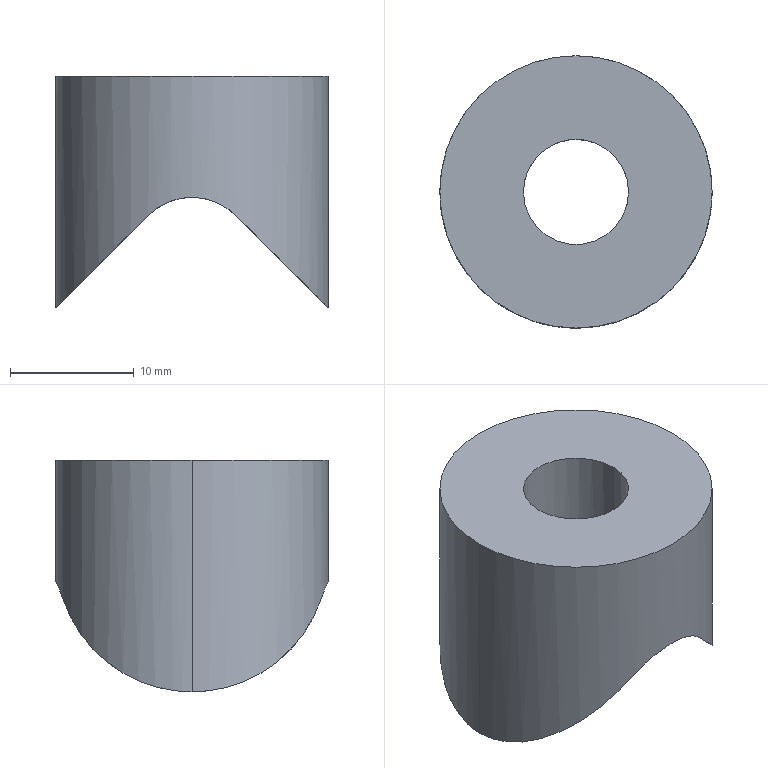Part | SolidWorks | features Extrusion 1, HoleWzd 1, ICE 1 | 1 solid | 11 faces | box 22 x 22 x 18.716 mm | volume 4241 mm3 | cylinder 8 | plane 3 | commonest cylinder face diameters 10 x4 8.5 x2 22 x2
STEP:
#1=CARTESIAN_POINT('',(0.,-11.,9.213));
#2=VERTEX_POINT('',#1);
#3=CARTESIAN_POINT('',(3.536,-10.416,7.749));
#4=VERTEX_POINT('',#3);
#5=CARTESIAN_POINT('',(0.,-11.,9.213));
#6=CARTESIAN_POINT('',(0.33,-11.,9.213));
#7=CARTESIAN_POINT('',(0.6582,-10.985,9.181));
#8=CARTESIAN_POINT('',(1.311,-10.927,9.05));
#9=CARTESIAN_POINT('',(1.625,-10.884,8.953));
#10=CARTESIAN_POINT('',(2.227,-10.776,8.702));
#11=CARTESIAN_POINT('',(2.518,-10.712,8.545));
#12=CARTESIAN_POINT('',(3.056,-10.571,8.184));
#13=CARTESIAN_POINT('',(3.306,-10.494,7.979));
#14=CARTESIAN_POINT('',(3.536,-10.416,7.749));
#15=B_SPLINE_CURVE_WITH_KNOTS('',3,(#5,#6,#7,#8,#9,#10,#11,#12,#13,#14),.UNSPECIFIED.,.F.,.F.,(4,2,2,2,4),(0.003963,0.004952,0.005942,0.006931,0.00792),.UNSPECIFIED.);
#16=EDGE_CURVE('',#2,#4,#15,.T.);
#17=ORIENTED_EDGE('',*,*,#16,.F.);
#18=CARTESIAN_POINT('',(0.,-4.25,9.213));
#19=VERTEX_POINT('',#18);
#20=CARTESIAN_POINT('',(0.,-12.5,9.213));
#21=DIRECTION('',(0.,1.,0.));
#22=VECTOR('',#21,1000.);
#23=LINE('',#20,#22);
#24=EDGE_CURVE('',#2,#19,#23,.T.);
#25=ORIENTED_EDGE('',*,*,#24,.T.);
#26=CARTESIAN_POINT('',(3.536,-2.358,7.749));
#27=VERTEX_POINT('',#26);
#28=CARTESIAN_POINT('',(3.536,-2.358,7.749));
#29=CARTESIAN_POINT('',(3.353,-2.632,7.931));
#30=CARTESIAN_POINT('',(3.144,-2.879,8.113));
#31=CARTESIAN_POINT('',(2.663,-3.329,8.456));
#32=CARTESIAN_POINT('',(2.387,-3.533,8.619));
#33=CARTESIAN_POINT('',(1.936,-3.787,8.826));
#34=CARTESIAN_POINT('',(1.779,-3.864,8.889));
#35=CARTESIAN_POINT('',(1.449,-3.999,9.002));
#36=CARTESIAN_POINT('',(1.276,-4.058,9.051));
#37=CARTESIAN_POINT('',(0.9236,-4.152,9.13));
#38=CARTESIAN_POINT('',(0.7437,-4.189,9.161));
#39=CARTESIAN_POINT('',(0.376,-4.237,9.202));
#40=CARTESIAN_POINT('',(0.1866,-4.25,9.213));
#41=CARTESIAN_POINT('',(0.,-4.25,9.213));
#42=B_SPLINE_CURVE_WITH_KNOTS('',3,(#28,#29,#30,#31,#32,#33,#34,#35,#36,#37,#38,#39,#40,#41),.UNSPECIFIED.,.F.,.F.,(4,2,2,2,2,2,4),(0.,0.001113,0.002226,0.002782,0.003338,0.003895,0.004451),.UNSPECIFIED.);
#43=EDGE_CURVE('',#27,#19,#42,.T.);
#44=ORIENTED_EDGE('',*,*,#43,.F.);
#45=CARTESIAN_POINT('',(3.536,-12.5,7.749));
#46=DIRECTION('',(0.,1.,0.));
#47=VECTOR('',#46,1000.);
#48=LINE('',#45,#47);
#49=EDGE_CURVE('',#4,#27,#48,.T.);
#50=ORIENTED_EDGE('',*,*,#49,.F.);
#51=EDGE_LOOP('',(#17,#25,#44,#50));
#52=FACE_OUTER_BOUND('',#51,.T.);
#53=CARTESIAN_POINT('',(0.,-12.5,4.213));
#54=DIRECTION('',(0.,1.,0.));
#55=DIRECTION('',(0.,0.,1.));
#56=AXIS2_PLACEMENT_3D('',#53,#54,#55);
#57=CYLINDRICAL_SURFACE('',#56,5.);
#58=ADVANCED_FACE('',(#52),#57,.F.);
#59=CARTESIAN_POINT('',(0.,4.25,9.213));
#60=VERTEX_POINT('',#59);
#61=CARTESIAN_POINT('',(3.536,2.358,7.749));
#62=VERTEX_POINT('',#61);
#63=CARTESIAN_POINT('',(0.,4.25,9.213));
#64=CARTESIAN_POINT('',(0.1864,4.25,9.213));
#65=CARTESIAN_POINT('',(0.3713,4.238,9.203));
#66=CARTESIAN_POINT('',(0.7382,4.189,9.162));
#67=CARTESIAN_POINT('',(0.9217,4.153,9.131));
#68=CARTESIAN_POINT('',(1.274,4.059,9.051));
#69=CARTESIAN_POINT('',(1.445,4.001,9.003));
#70=CARTESIAN_POINT('',(1.774,3.866,8.891));
#71=CARTESIAN_POINT('',(1.934,3.788,8.827));
#72=CARTESIAN_POINT('',(2.387,3.533,8.619));
#73=CARTESIAN_POINT('',(2.656,3.334,8.46));
#74=CARTESIAN_POINT('',(3.141,2.882,8.115));
#75=CARTESIAN_POINT('',(3.353,2.632,7.931));
#76=CARTESIAN_POINT('',(3.536,2.358,7.749));
#77=B_SPLINE_CURVE_WITH_KNOTS('',3,(#63,#64,#65,#66,#67,#68,#69,#70,#71,#72,#73,#74,#75,#76),.UNSPECIFIED.,.F.,.F.,(4,2,2,2,2,2,4),(0.004451,0.005007,0.005562,0.006118,0.006674,0.007785,0.008897),.UNSPECIFIED.);
#78=EDGE_CURVE('',#60,#62,#77,.T.);
#79=ORIENTED_EDGE('',*,*,#78,.F.);
#80=CARTESIAN_POINT('',(0.,11.,9.213));
#81=VERTEX_POINT('',#80);
#82=CARTESIAN_POINT('',(0.,-12.5,9.213));
#83=DIRECTION('',(0.,1.,0.));
#84=VECTOR('',#83,1000.);
#85=LINE('',#82,#84);
#86=EDGE_CURVE('',#60,#81,#85,.T.);
#87=ORIENTED_EDGE('',*,*,#86,.T.);
#88=CARTESIAN_POINT('',(3.536,10.416,7.749));
#89=VERTEX_POINT('',#88);
#90=CARTESIAN_POINT('',(3.536,10.416,7.749));
#91=CARTESIAN_POINT('',(3.305,10.494,7.979));
#92=CARTESIAN_POINT('',(3.056,10.57,8.183));
#93=CARTESIAN_POINT('',(2.655,10.676,8.453));
#94=CARTESIAN_POINT('',(2.516,10.709,8.537));
#95=CARTESIAN_POINT('',(2.228,10.773,8.692));
#96=CARTESIAN_POINT('',(2.079,10.803,8.764));
#97=CARTESIAN_POINT('',(1.625,10.884,8.953));
#98=CARTESIAN_POINT('',(1.313,10.926,9.049));
#99=CARTESIAN_POINT('',(0.6667,10.985,9.18));
#100=CARTESIAN_POINT('',(0.3305,11.,9.213));
#101=CARTESIAN_POINT('',(0.,11.,9.213));
#102=B_SPLINE_CURVE_WITH_KNOTS('',3,(#90,#91,#92,#93,#94,#95,#96,#97,#98,#99,#100,#101),.UNSPECIFIED.,.F.,.F.,(4,2,2,2,2,4),(0.,0.0009907,0.001486,0.001981,0.002972,0.003963),.UNSPECIFIED.);
#103=EDGE_CURVE('',#89,#81,#102,.T.);
#104=ORIENTED_EDGE('',*,*,#103,.F.);
#105=CARTESIAN_POINT('',(3.536,-12.5,7.749));
#106=DIRECTION('',(0.,1.,0.));
#107=VECTOR('',#106,1000.);
#108=LINE('',#105,#107);
#109=EDGE_CURVE('',#62,#89,#108,.T.);
#110=ORIENTED_EDGE('',*,*,#109,.F.);
#111=EDGE_LOOP('',(#79,#87,#104,#110));
#112=FACE_OUTER_BOUND('',#111,.T.);
#113=CARTESIAN_POINT('',(0.,-12.5,4.213));
#114=DIRECTION('',(0.,1.,0.));
#115=DIRECTION('',(0.,0.,1.));
#116=AXIS2_PLACEMENT_3D('',#113,#114,#115);
#117=CYLINDRICAL_SURFACE('',#116,5.);
#118=ADVANCED_FACE('',(#112),#117,.F.);
#119=CARTESIAN_POINT('',(-3.536,-2.358,7.749));
#120=VERTEX_POINT('',#119);
#121=CARTESIAN_POINT('',(-4.25,0.,7.034));
#122=VERTEX_POINT('',#121);
#123=CARTESIAN_POINT('',(-3.536,-2.358,7.749));
#124=CARTESIAN_POINT('',(-4.005,-1.655,7.279));
#125=CARTESIAN_POINT('',(-4.25,-0.8457,7.034));
#126=CARTESIAN_POINT('',(-4.25,0.,7.034));
#127=(BOUNDED_CURVE()B_SPLINE_CURVE(3,(#123,#124,#125,#126),.UNSPECIFIED.,.F.,.F.)B_SPLINE_CURVE_WITH_KNOTS((4,4),(2.553,3.142),.UNSPECIFIED.)CURVE()GEOMETRIC_REPRESENTATION_ITEM()RATIONAL_B_SPLINE_CURVE((1.,0.9714,0.9714,1.))REPRESENTATION_ITEM(''));
#128=EDGE_CURVE('',#120,#122,#127,.T.);
#129=ORIENTED_EDGE('',*,*,#128,.T.);
#130=CARTESIAN_POINT('',(-4.25,0.,19.));
#131=VERTEX_POINT('',#130);
#132=CARTESIAN_POINT('',(-4.25,0.,19.));
#133=DIRECTION('',(0.,0.,1.));
#134=VECTOR('',#133,1000.);
#135=LINE('',#132,#134);
#136=EDGE_CURVE('',#122,#131,#135,.T.);
#137=ORIENTED_EDGE('',*,*,#136,.T.);
#138=CARTESIAN_POINT('',(4.25,0.,19.));
#139=VERTEX_POINT('',#138);
#140=CARTESIAN_POINT('',(0.,0.,19.));
#141=DIRECTION('',(0.,0.,1.));
#142=DIRECTION('',(1.,0.,0.));
#143=AXIS2_PLACEMENT_3D('',#140,#141,#142);
#144=CIRCLE('',#143,4.25);
#145=EDGE_CURVE('',#131,#139,#144,.T.);
#146=ORIENTED_EDGE('',*,*,#145,.T.);
#147=CARTESIAN_POINT('',(4.25,0.,7.034));
#148=VERTEX_POINT('',#147);
#149=CARTESIAN_POINT('',(4.25,0.,19.));
#150=DIRECTION('',(0.,0.,1.));
#151=VECTOR('',#150,1000.);
#152=LINE('',#149,#151);
#153=EDGE_CURVE('',#148,#139,#152,.T.);
#154=ORIENTED_EDGE('',*,*,#153,.F.);
#155=CARTESIAN_POINT('',(4.25,0.,7.034));
#156=CARTESIAN_POINT('',(4.25,-0.8457,7.034));
#157=CARTESIAN_POINT('',(4.005,-1.655,7.279));
#158=CARTESIAN_POINT('',(3.536,-2.358,7.749));
#159=(BOUNDED_CURVE()B_SPLINE_CURVE(3,(#155,#156,#157,#158),.UNSPECIFIED.,.F.,.F.)B_SPLINE_CURVE_WITH_KNOTS((4,4),(3.142,3.73),.UNSPECIFIED.)CURVE()GEOMETRIC_REPRESENTATION_ITEM()RATIONAL_B_SPLINE_CURVE((1.,0.9714,0.9714,1.))REPRESENTATION_ITEM(''));
#160=EDGE_CURVE('',#148,#27,#159,.T.);
#161=ORIENTED_EDGE('',*,*,#160,.T.);
#162=ORIENTED_EDGE('',*,*,#43,.T.);
#163=CARTESIAN_POINT('',(0.,-4.25,9.213));
#164=CARTESIAN_POINT('',(-0.1864,-4.25,9.213));
#165=CARTESIAN_POINT('',(-0.3713,-4.238,9.203));
#166=CARTESIAN_POINT('',(-0.7382,-4.189,9.162));
#167=CARTESIAN_POINT('',(-0.9217,-4.153,9.131));
#168=CARTESIAN_POINT('',(-1.274,-4.059,9.051));
#169=CARTESIAN_POINT('',(-1.445,-4.001,9.003));
#170=CARTESIAN_POINT('',(-1.774,-3.866,8.891));
#171=CARTESIAN_POINT('',(-1.934,-3.788,8.827));
#172=CARTESIAN_POINT('',(-2.387,-3.533,8.619));
#173=CARTESIAN_POINT('',(-2.656,-3.334,8.46));
#174=CARTESIAN_POINT('',(-3.141,-2.882,8.115));
#175=CARTESIAN_POINT('',(-3.353,-2.632,7.931));
#176=CARTESIAN_POINT('',(-3.536,-2.358,7.749));
#177=B_SPLINE_CURVE_WITH_KNOTS('',3,(#163,#164,#165,#166,#167,#168,#169,#170,#171,#172,#173,#174,#175,#176),.UNSPECIFIED.,.F.,.F.,(4,2,2,2,2,2,4),(0.004451,0.005007,0.005562,0.006118,0.006674,0.007785,0.008897),.UNSPECIFIED.);
#178=EDGE_CURVE('',#19,#120,#177,.T.);
#179=ORIENTED_EDGE('',*,*,#178,.T.);
#180=EDGE_LOOP('',(#129,#137,#146,#154,#161,#162,#179));
#181=FACE_OUTER_BOUND('',#180,.T.);
#182=CARTESIAN_POINT('',(0.,0.,19.));
#183=DIRECTION('',(0.,0.,1.));
#184=DIRECTION('',(1.,0.,0.));
#185=AXIS2_PLACEMENT_3D('',#182,#183,#184);
#186=CYLINDRICAL_SURFACE('',#185,4.25);
#187=ADVANCED_FACE('',(#181),#186,.F.);
#188=CARTESIAN_POINT('',(11.,0.,19.));
#189=VERTEX_POINT('',#188);
#190=CARTESIAN_POINT('',(-11.,0.,19.));
#191=VERTEX_POINT('',#190);
#192=CARTESIAN_POINT('',(0.,0.,19.));
#193=DIRECTION('',(0.,0.,1.));
#194=DIRECTION('',(1.,0.,0.));
#195=AXIS2_PLACEMENT_3D('',#192,#193,#194);
#196=CIRCLE('',#195,11.);
#197=EDGE_CURVE('',#189,#191,#196,.T.);
#198=ORIENTED_EDGE('',*,*,#197,.F.);
#199=CARTESIAN_POINT('',(11.,0.,0.2843));
#200=VERTEX_POINT('',#199);
#201=CARTESIAN_POINT('',(11.,0.,19.));
#202=DIRECTION('',(0.,0.,-1.));
#203=VECTOR('',#202,1000.);
#204=LINE('',#201,#203);
#205=EDGE_CURVE('',#189,#200,#204,.T.);
#206=ORIENTED_EDGE('',*,*,#205,.T.);
#207=CARTESIAN_POINT('',(11.,0.,0.2843));
#208=CARTESIAN_POINT('',(11.,4.881,0.2843));
#209=CARTESIAN_POINT('',(8.157,8.848,3.127));
#210=CARTESIAN_POINT('',(3.536,10.416,7.749));
#211=(BOUNDED_CURVE()B_SPLINE_CURVE(3,(#207,#208,#209,#210),.UNSPECIFIED.,.F.,.F.)B_SPLINE_CURVE_WITH_KNOTS((4,4),(0.,1.244),.UNSPECIFIED.)CURVE()GEOMETRIC_REPRESENTATION_ITEM()RATIONAL_B_SPLINE_CURVE((1.,0.8752,0.8752,1.))REPRESENTATION_ITEM(''));
#212=EDGE_CURVE('',#200,#89,#211,.T.);
#213=ORIENTED_EDGE('',*,*,#212,.T.);
#214=ORIENTED_EDGE('',*,*,#103,.T.);
#215=CARTESIAN_POINT('',(-3.536,10.416,7.749));
#216=VERTEX_POINT('',#215);
#217=CARTESIAN_POINT('',(0.,11.,9.213));
#218=CARTESIAN_POINT('',(-0.33,11.,9.213));
#219=CARTESIAN_POINT('',(-0.6582,10.985,9.181));
#220=CARTESIAN_POINT('',(-1.311,10.927,9.05));
#221=CARTESIAN_POINT('',(-1.625,10.884,8.953));
#222=CARTESIAN_POINT('',(-2.227,10.776,8.702));
#223=CARTESIAN_POINT('',(-2.518,10.712,8.545));
#224=CARTESIAN_POINT('',(-3.056,10.571,8.184));
#225=CARTESIAN_POINT('',(-3.306,10.494,7.979));
#226=CARTESIAN_POINT('',(-3.536,10.416,7.749));
#227=B_SPLINE_CURVE_WITH_KNOTS('',3,(#217,#218,#219,#220,#221,#222,#223,#224,#225,#226),.UNSPECIFIED.,.F.,.F.,(4,2,2,2,4),(0.003963,0.004952,0.005942,0.006931,0.00792),.UNSPECIFIED.);
#228=EDGE_CURVE('',#81,#216,#227,.T.);
#229=ORIENTED_EDGE('',*,*,#228,.T.);
#230=CARTESIAN_POINT('',(-11.,0.,0.2843));
#231=VERTEX_POINT('',#230);
#232=CARTESIAN_POINT('',(-3.536,10.416,7.749));
#233=CARTESIAN_POINT('',(-8.157,8.848,3.127));
#234=CARTESIAN_POINT('',(-11.,4.881,0.2843));
#235=CARTESIAN_POINT('',(-11.,0.,0.2843));
#236=(BOUNDED_CURVE()B_SPLINE_CURVE(3,(#232,#233,#234,#235),.UNSPECIFIED.,.F.,.T.)B_SPLINE_CURVE_WITH_KNOTS((4,4),(5.04,6.283),.UNSPECIFIED.)CURVE()GEOMETRIC_REPRESENTATION_ITEM()RATIONAL_B_SPLINE_CURVE((1.,0.8752,0.8752,1.))REPRESENTATION_ITEM(''));
#237=EDGE_CURVE('',#216,#231,#236,.T.);
#238=ORIENTED_EDGE('',*,*,#237,.T.);
#239=CARTESIAN_POINT('',(-11.,0.,19.));
#240=DIRECTION('',(0.,0.,-1.));
#241=VECTOR('',#240,1000.);
#242=LINE('',#239,#241);
#243=EDGE_CURVE('',#191,#231,#242,.T.);
#244=ORIENTED_EDGE('',*,*,#243,.F.);
#245=EDGE_LOOP('',(#198,#206,#213,#214,#229,#238,#244));
#246=FACE_OUTER_BOUND('',#245,.T.);
#247=CARTESIAN_POINT('',(0.,0.,19.));
#248=DIRECTION('',(0.,0.,-1.));
#249=DIRECTION('',(-1.,0.,0.));
#250=AXIS2_PLACEMENT_3D('',#247,#248,#249);
#251=CYLINDRICAL_SURFACE('',#250,11.);
#252=ADVANCED_FACE('',(#246),#251,.T.);
#253=ORIENTED_EDGE('',*,*,#205,.F.);
#254=CARTESIAN_POINT('',(0.,0.,19.));
#255=DIRECTION('',(0.,0.,1.));
#256=DIRECTION('',(1.,0.,0.));
#257=AXIS2_PLACEMENT_3D('',#254,#255,#256);
#258=CIRCLE('',#257,11.);
#259=EDGE_CURVE('',#191,#189,#258,.T.);
#260=ORIENTED_EDGE('',*,*,#259,.F.);
#261=ORIENTED_EDGE('',*,*,#243,.T.);
#262=CARTESIAN_POINT('',(-3.536,-10.416,7.749));
#263=VERTEX_POINT('',#262);
#264=CARTESIAN_POINT('',(-11.,0.,0.2843));
#265=CARTESIAN_POINT('',(-11.,-4.881,0.2843));
#266=CARTESIAN_POINT('',(-8.157,-8.848,3.127));
#267=CARTESIAN_POINT('',(-3.536,-10.416,7.749));
#268=(BOUNDED_CURVE()B_SPLINE_CURVE(3,(#264,#265,#266,#267),.UNSPECIFIED.,.F.,.F.)B_SPLINE_CURVE_WITH_KNOTS((4,4),(0.,1.244),.UNSPECIFIED.)CURVE()GEOMETRIC_REPRESENTATION_ITEM()RATIONAL_B_SPLINE_CURVE((1.,0.8752,0.8752,1.))REPRESENTATION_ITEM(''));
#269=EDGE_CURVE('',#231,#263,#268,.T.);
#270=ORIENTED_EDGE('',*,*,#269,.T.);
#271=CARTESIAN_POINT('',(-3.536,-10.416,7.749));
#272=CARTESIAN_POINT('',(-3.305,-10.494,7.979));
#273=CARTESIAN_POINT('',(-3.056,-10.57,8.183));
#274=CARTESIAN_POINT('',(-2.655,-10.676,8.453));
#275=CARTESIAN_POINT('',(-2.516,-10.709,8.537));
#276=CARTESIAN_POINT('',(-2.228,-10.773,8.692));
#277=CARTESIAN_POINT('',(-2.079,-10.803,8.764));
#278=CARTESIAN_POINT('',(-1.625,-10.884,8.953));
#279=CARTESIAN_POINT('',(-1.313,-10.926,9.049));
#280=CARTESIAN_POINT('',(-0.6667,-10.985,9.18));
#281=CARTESIAN_POINT('',(-0.3305,-11.,9.213));
#282=CARTESIAN_POINT('',(0.,-11.,9.213));
#283=B_SPLINE_CURVE_WITH_KNOTS('',3,(#271,#272,#273,#274,#275,#276,#277,#278,#279,#280,#281,#282),.UNSPECIFIED.,.F.,.F.,(4,2,2,2,2,4),(0.,0.0009907,0.001486,0.001981,0.002972,0.003963),.UNSPECIFIED.);
#284=EDGE_CURVE('',#263,#2,#283,.T.);
#285=ORIENTED_EDGE('',*,*,#284,.T.);
#286=ORIENTED_EDGE('',*,*,#16,.T.);
#287=CARTESIAN_POINT('',(3.536,-10.416,7.749));
#288=CARTESIAN_POINT('',(8.157,-8.848,3.127));
#289=CARTESIAN_POINT('',(11.,-4.881,0.2843));
#290=CARTESIAN_POINT('',(11.,0.,0.2843));
#291=(BOUNDED_CURVE()B_SPLINE_CURVE(3,(#287,#288,#289,#290),.UNSPECIFIED.,.F.,.T.)B_SPLINE_CURVE_WITH_KNOTS((4,4),(5.04,6.283),.UNSPECIFIED.)CURVE()GEOMETRIC_REPRESENTATION_ITEM()RATIONAL_B_SPLINE_CURVE((1.,0.8752,0.8752,1.))REPRESENTATION_ITEM(''));
#292=EDGE_CURVE('',#4,#200,#291,.T.);
#293=ORIENTED_EDGE('',*,*,#292,.T.);
#294=EDGE_LOOP('',(#253,#260,#261,#270,#285,#286,#293));
#295=FACE_OUTER_BOUND('',#294,.T.);
#296=CARTESIAN_POINT('',(0.,0.,19.));
#297=DIRECTION('',(0.,0.,-1.));
#298=DIRECTION('',(-1.,0.,0.));
#299=AXIS2_PLACEMENT_3D('',#296,#297,#298);
#300=CYLINDRICAL_SURFACE('',#299,11.);
#301=ADVANCED_FACE('',(#295),#300,.T.);
#302=CARTESIAN_POINT('',(0.,0.,19.));
#303=DIRECTION('',(0.,0.,1.));
#304=DIRECTION('',(1.,0.,0.));
#305=AXIS2_PLACEMENT_3D('',#302,#303,#304);
#306=CIRCLE('',#305,4.25);
#307=EDGE_CURVE('',#139,#131,#306,.T.);
#308=ORIENTED_EDGE('',*,*,#307,.F.);
#309=ORIENTED_EDGE('',*,*,#145,.F.);
#310=EDGE_LOOP('',(#308,#309));
#311=FACE_BOUND('',#310,.T.);
#312=ORIENTED_EDGE('',*,*,#259,.T.);
#313=ORIENTED_EDGE('',*,*,#197,.T.);
#314=EDGE_LOOP('',(#312,#313));
#315=FACE_OUTER_BOUND('',#314,.T.);
#316=CARTESIAN_POINT('',(0.,0.,19.));
#317=DIRECTION('',(0.,0.,1.));
#318=DIRECTION('',(1.,0.,0.));
#319=AXIS2_PLACEMENT_3D('',#316,#317,#318);
#320=PLANE('',#319);
#321=ADVANCED_FACE('',(#311,#315),#320,.T.);
#322=ORIENTED_EDGE('',*,*,#136,.F.);
#323=CARTESIAN_POINT('',(-3.536,2.358,7.749));
#324=VERTEX_POINT('',#323);
#325=CARTESIAN_POINT('',(-4.25,0.,7.034));
#326=CARTESIAN_POINT('',(-4.25,0.8457,7.034));
#327=CARTESIAN_POINT('',(-4.005,1.655,7.279));
#328=CARTESIAN_POINT('',(-3.536,2.358,7.749));
#329=(BOUNDED_CURVE()B_SPLINE_CURVE(3,(#325,#326,#327,#328),.UNSPECIFIED.,.F.,.F.)B_SPLINE_CURVE_WITH_KNOTS((4,4),(3.142,3.73),.UNSPECIFIED.)CURVE()GEOMETRIC_REPRESENTATION_ITEM()RATIONAL_B_SPLINE_CURVE((1.,0.9714,0.9714,1.))REPRESENTATION_ITEM(''));
#330=EDGE_CURVE('',#122,#324,#329,.T.);
#331=ORIENTED_EDGE('',*,*,#330,.T.);
#332=CARTESIAN_POINT('',(-3.536,2.358,7.749));
#333=CARTESIAN_POINT('',(-3.353,2.632,7.931));
#334=CARTESIAN_POINT('',(-3.144,2.879,8.113));
#335=CARTESIAN_POINT('',(-2.663,3.329,8.456));
#336=CARTESIAN_POINT('',(-2.387,3.533,8.619));
#337=CARTESIAN_POINT('',(-1.936,3.787,8.826));
#338=CARTESIAN_POINT('',(-1.779,3.864,8.889));
#339=CARTESIAN_POINT('',(-1.449,3.999,9.002));
#340=CARTESIAN_POINT('',(-1.276,4.058,9.051));
#341=CARTESIAN_POINT('',(-0.9236,4.152,9.13));
#342=CARTESIAN_POINT('',(-0.7437,4.189,9.161));
#343=CARTESIAN_POINT('',(-0.376,4.237,9.202));
#344=CARTESIAN_POINT('',(-0.1866,4.25,9.213));
#345=CARTESIAN_POINT('',(0.,4.25,9.213));
#346=B_SPLINE_CURVE_WITH_KNOTS('',3,(#332,#333,#334,#335,#336,#337,#338,#339,#340,#341,#342,#343,#344,#345),.UNSPECIFIED.,.F.,.F.,(4,2,2,2,2,2,4),(0.,0.001113,0.002226,0.002782,0.003338,0.003895,0.004451),.UNSPECIFIED.);
#347=EDGE_CURVE('',#324,#60,#346,.T.);
#348=ORIENTED_EDGE('',*,*,#347,.T.);
#349=ORIENTED_EDGE('',*,*,#78,.T.);
#350=CARTESIAN_POINT('',(3.536,2.358,7.749));
#351=CARTESIAN_POINT('',(4.005,1.655,7.279));
#352=CARTESIAN_POINT('',(4.25,0.8457,7.034));
#353=CARTESIAN_POINT('',(4.25,0.,7.034));
#354=(BOUNDED_CURVE()B_SPLINE_CURVE(3,(#350,#351,#352,#353),.UNSPECIFIED.,.F.,.F.)B_SPLINE_CURVE_WITH_KNOTS((4,4),(2.553,3.142),.UNSPECIFIED.)CURVE()GEOMETRIC_REPRESENTATION_ITEM()RATIONAL_B_SPLINE_CURVE((1.,0.9714,0.9714,1.))REPRESENTATION_ITEM(''));
#355=EDGE_CURVE('',#62,#148,#354,.T.);
#356=ORIENTED_EDGE('',*,*,#355,.T.);
#357=ORIENTED_EDGE('',*,*,#153,.T.);
#358=ORIENTED_EDGE('',*,*,#307,.T.);
#359=EDGE_LOOP('',(#322,#331,#348,#349,#356,#357,#358));
#360=FACE_OUTER_BOUND('',#359,.T.);
#361=CARTESIAN_POINT('',(0.,0.,19.));
#362=DIRECTION('',(0.,0.,1.));
#363=DIRECTION('',(1.,0.,0.));
#364=AXIS2_PLACEMENT_3D('',#361,#362,#363);
#365=CYLINDRICAL_SURFACE('',#364,4.25);
#366=ADVANCED_FACE('',(#360),#365,.F.);
#367=ORIENTED_EDGE('',*,*,#49,.T.);
#368=ORIENTED_EDGE('',*,*,#160,.F.);
#369=ORIENTED_EDGE('',*,*,#355,.F.);
#370=ORIENTED_EDGE('',*,*,#109,.T.);
#371=ORIENTED_EDGE('',*,*,#212,.F.);
#372=ORIENTED_EDGE('',*,*,#292,.F.);
#373=EDGE_LOOP('',(#367,#368,#369,#370,#371,#372));
#374=FACE_OUTER_BOUND('',#373,.T.);
#375=CARTESIAN_POINT('',(3.536,-12.5,7.749));
#376=DIRECTION('',(0.7071,0.,0.7071));
#377=DIRECTION('',(0.7071,0.,-0.7071));
#378=AXIS2_PLACEMENT_3D('',#375,#376,#377);
#379=PLANE('',#378);
#380=ADVANCED_FACE('',(#374),#379,.F.);
#381=ORIENTED_EDGE('',*,*,#86,.F.);
#382=ORIENTED_EDGE('',*,*,#347,.F.);
#383=CARTESIAN_POINT('',(-3.536,-12.5,7.749));
#384=DIRECTION('',(0.,1.,0.));
#385=VECTOR('',#384,1000.);
#386=LINE('',#383,#385);
#387=EDGE_CURVE('',#324,#216,#386,.T.);
#388=ORIENTED_EDGE('',*,*,#387,.T.);
#389=ORIENTED_EDGE('',*,*,#228,.F.);
#390=EDGE_LOOP('',(#381,#382,#388,#389));
#391=FACE_OUTER_BOUND('',#390,.T.);
#392=CARTESIAN_POINT('',(0.,-12.5,4.213));
#393=DIRECTION('',(0.,1.,0.));
#394=DIRECTION('',(0.,0.,1.));
#395=AXIS2_PLACEMENT_3D('',#392,#393,#394);
#396=CYLINDRICAL_SURFACE('',#395,5.);
#397=ADVANCED_FACE('',(#391),#396,.F.);
#398=ORIENTED_EDGE('',*,*,#24,.F.);
#399=ORIENTED_EDGE('',*,*,#284,.F.);
#400=CARTESIAN_POINT('',(-3.536,-12.5,7.749));
#401=DIRECTION('',(0.,1.,0.));
#402=VECTOR('',#401,1000.);
#403=LINE('',#400,#402);
#404=EDGE_CURVE('',#263,#120,#403,.T.);
#405=ORIENTED_EDGE('',*,*,#404,.T.);
#406=ORIENTED_EDGE('',*,*,#178,.F.);
#407=EDGE_LOOP('',(#398,#399,#405,#406));
#408=FACE_OUTER_BOUND('',#407,.T.);
#409=CARTESIAN_POINT('',(0.,-12.5,4.213));
#410=DIRECTION('',(0.,1.,0.));
#411=DIRECTION('',(0.,0.,1.));
#412=AXIS2_PLACEMENT_3D('',#409,#410,#411);
#413=CYLINDRICAL_SURFACE('',#412,5.);
#414=ADVANCED_FACE('',(#408),#413,.F.);
#415=ORIENTED_EDGE('',*,*,#387,.F.);
#416=ORIENTED_EDGE('',*,*,#330,.F.);
#417=ORIENTED_EDGE('',*,*,#128,.F.);
#418=ORIENTED_EDGE('',*,*,#404,.F.);
#419=ORIENTED_EDGE('',*,*,#269,.F.);
#420=ORIENTED_EDGE('',*,*,#237,.F.);
#421=EDGE_LOOP('',(#415,#416,#417,#418,#419,#420));
#422=FACE_OUTER_BOUND('',#421,.T.);
#423=CARTESIAN_POINT('',(-3.536,-12.5,7.749));
#424=DIRECTION('',(-0.7071,0.,0.7071));
#425=DIRECTION('',(0.7071,0.,0.7071));
#426=AXIS2_PLACEMENT_3D('',#423,#424,#425);
#427=PLANE('',#426);
#428=ADVANCED_FACE('',(#422),#427,.F.);
#429=CLOSED_SHELL('',(#58,#118,#187,#252,#301,#321,#366,#380,#397,#414,#428));
#430=MANIFOLD_SOLID_BREP('',#429);
#431=CARTESIAN_POINT('',(0.,0.,0.));
#432=DIRECTION('',(0.,0.,1.));
#433=DIRECTION('',(1.,0.,0.));
#434=AXIS2_PLACEMENT_3D('',#431,#432,#433);
#435=(LENGTH_UNIT()NAMED_UNIT(*)SI_UNIT(.MILLI.,.METRE.));
#436=UNCERTAINTY_MEASURE_WITH_UNIT(LENGTH_MEASURE(0.00001),#435,'','');
#437=(NAMED_UNIT(*)PLANE_ANGLE_UNIT()SI_UNIT($,.RADIAN.));
#438=(NAMED_UNIT(*)SI_UNIT($,.STERADIAN.)SOLID_ANGLE_UNIT());
#439=(GEOMETRIC_REPRESENTATION_CONTEXT(3)GLOBAL_UNCERTAINTY_ASSIGNED_CONTEXT((#436))GLOBAL_UNIT_ASSIGNED_CONTEXT((#435,#437,#438))REPRESENTATION_CONTEXT('',''));
#440=ADVANCED_BREP_SHAPE_REPRESENTATION('',(#430,#434),#439);